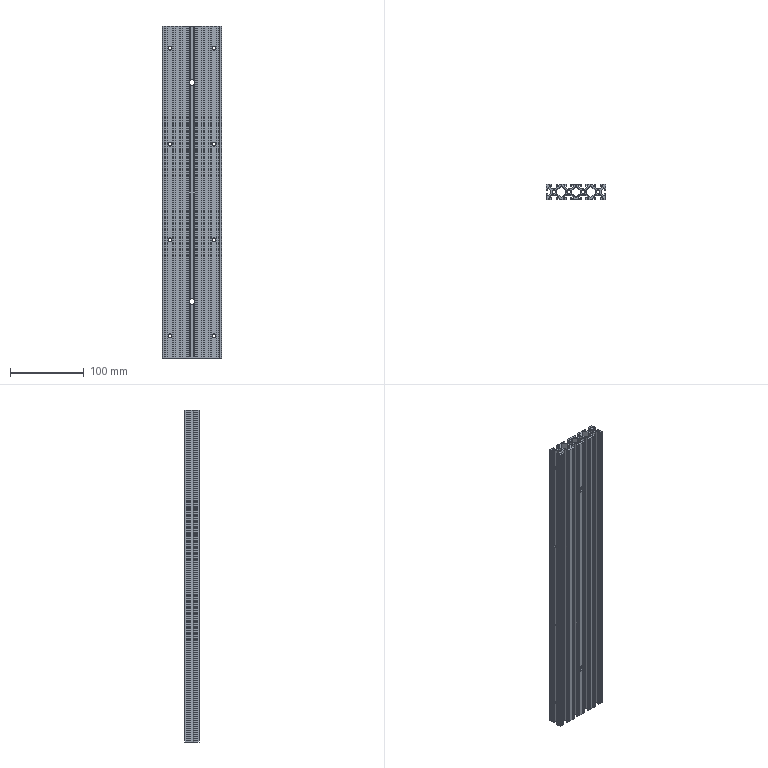Part | STEP file | 1 solid | 562 faces | box 80 x 20 x 450 mm | volume 285377 mm3 | plane 284 | cylinder 278 | commonest cylinder face diameters 0.2 x96 1 x88 10 x32 5 x24 5.5 x16 0.4 x14